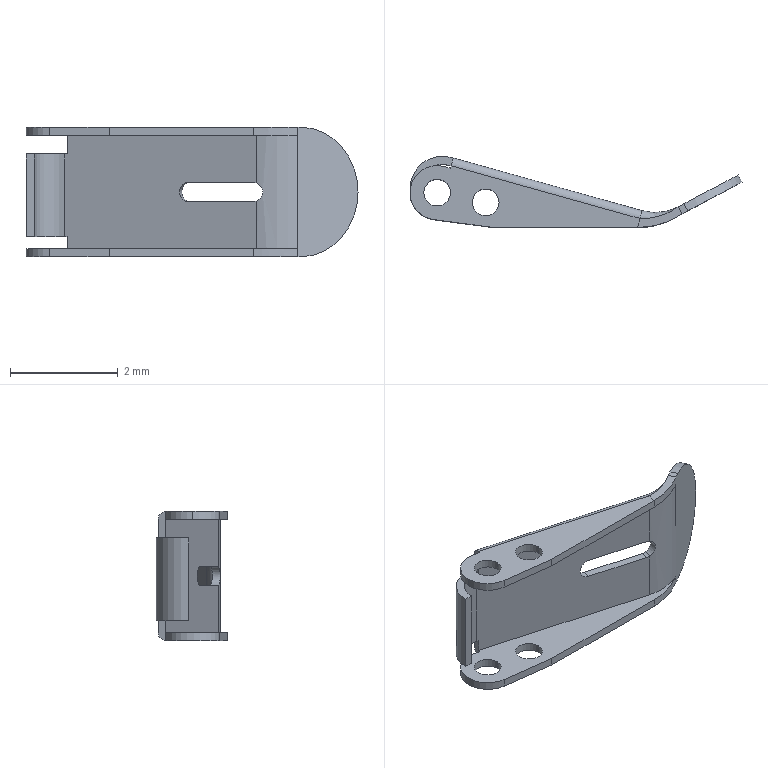Part | SolidWorks | features BaseBody 1, Scale 1 | 1 solid | 52 faces | box 6.154 x 1.321 x 2.4 mm | volume 2.823 mm3 | plane 23 | cylinder 22 | spline 7 | commonest cylinder face diameters 0.495 x8 0.36 x3 1.005 x3 0.3 x2 2.4 x2 0.9 x1